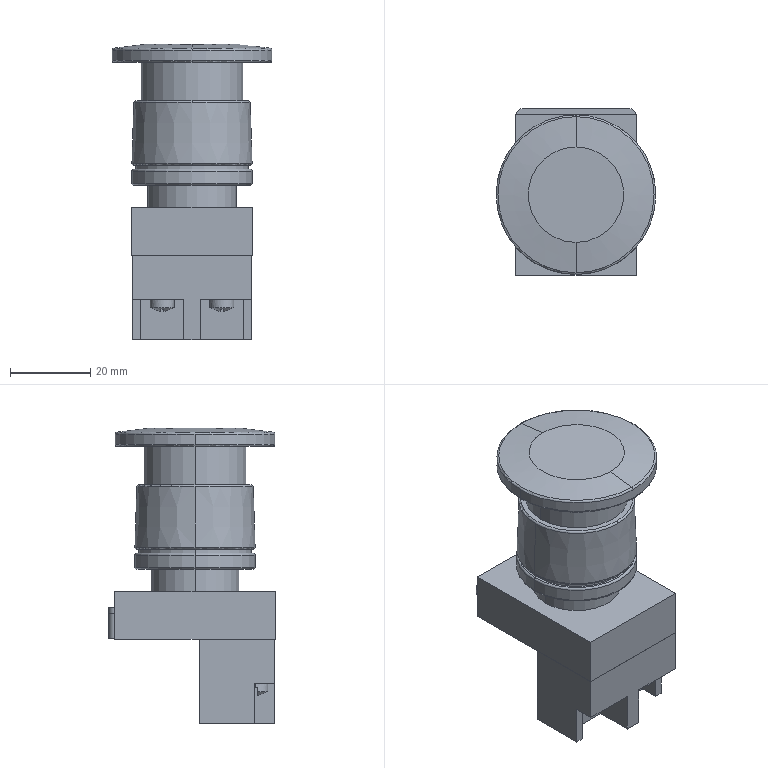Part | STEP file | Emergency stop | 1 solid | 100 faces | box 39.8 x 41.5 x 73.6 mm | volume 50842 mm3 | plane 62 | cylinder 18 | torus 12 | cone 8 | commonest cylinder face diameters 3 x4 6 x4 22 x2 25.4 x2 28 x2 30 x2